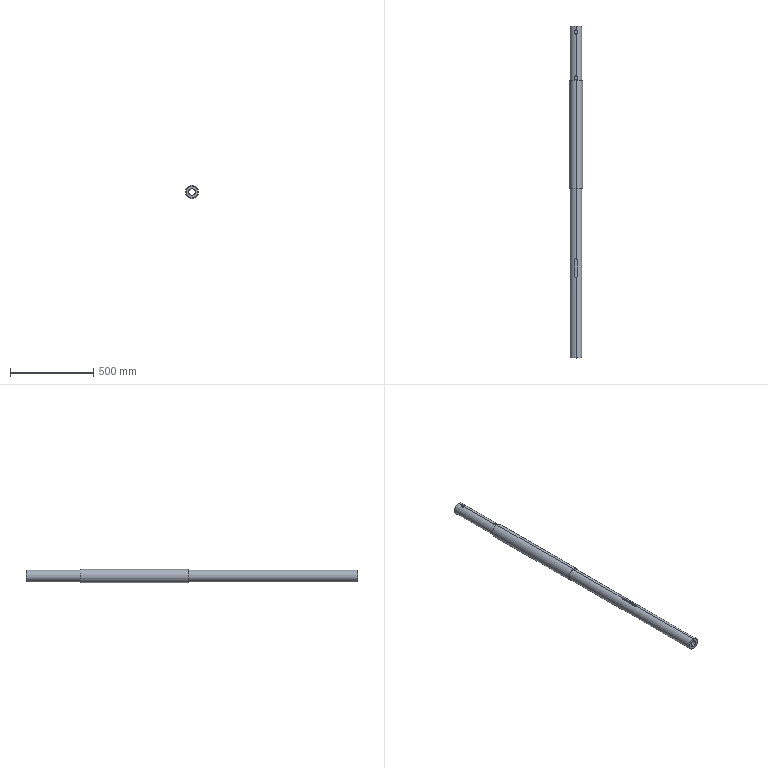Part | SolidWorks | features BaseBody 1 | 1 solid | 31 faces | box 80 x 1994 x 80 mm | volume 5902452 mm3 | cylinder 14 | plane 13 | cone 4 | commonest cylinder face diameters 14 x6 70 x4 40 x2 80 x2
STEP:
#1=CARTESIAN_POINT('',(0.,1994.06,-34.188));
#2=VERTEX_POINT('',#1);
#3=CARTESIAN_POINT('',(0.,1994.06,34.188));
#4=VERTEX_POINT('',#3);
#5=CARTESIAN_POINT('',(0.,1994.06,0.));
#6=DIRECTION('',(0.,-1.,0.));
#7=DIRECTION('',(0.,0.,-1.));
#8=AXIS2_PLACEMENT_3D('',#5,#6,#7);
#9=CIRCLE('',#8,34.188);
#10=EDGE_CURVE('',#2,#4,#9,.T.);
#11=ORIENTED_EDGE('',*,*,#10,.T.);
#12=CARTESIAN_POINT('',(0.,1993.248,35.));
#13=VERTEX_POINT('',#12);
#14=CARTESIAN_POINT('',(0.,1994.06,34.188));
#15=DIRECTION('',(0.,-0.7071,0.7071));
#16=VECTOR('',#15,1000.);
#17=LINE('',#14,#16);
#18=EDGE_CURVE('',#4,#13,#17,.T.);
#19=ORIENTED_EDGE('',*,*,#18,.T.);
#20=CARTESIAN_POINT('',(0.,1993.248,-35.));
#21=VERTEX_POINT('',#20);
#22=CARTESIAN_POINT('',(0.,1993.248,0.));
#23=DIRECTION('',(0.,-1.,0.));
#24=DIRECTION('',(0.,0.,-1.));
#25=AXIS2_PLACEMENT_3D('',#22,#23,#24);
#26=CIRCLE('',#25,35.);
#27=EDGE_CURVE('',#21,#13,#26,.T.);
#28=ORIENTED_EDGE('',*,*,#27,.F.);
#29=CARTESIAN_POINT('',(0.,1994.06,-34.188));
#30=DIRECTION('',(0.,-0.7071,-0.7071));
#31=VECTOR('',#30,1000.);
#32=LINE('',#29,#31);
#33=EDGE_CURVE('',#2,#21,#32,.T.);
#34=ORIENTED_EDGE('',*,*,#33,.F.);
#35=EDGE_LOOP('',(#11,#19,#28,#34));
#36=FACE_OUTER_BOUND('',#35,.T.);
#37=CARTESIAN_POINT('',(0.,1994.06,0.));
#38=DIRECTION('',(0.,-1.,0.));
#39=DIRECTION('',(0.,0.,-1.));
#40=AXIS2_PLACEMENT_3D('',#37,#38,#39);
#41=CONICAL_SURFACE('',#40,34.188,0.7854);
#42=ADVANCED_FACE('',(#36),#41,.T.);
#43=CARTESIAN_POINT('',(0.,0.,34.188));
#44=VERTEX_POINT('',#43);
#45=CARTESIAN_POINT('',(0.,0.,-34.188));
#46=VERTEX_POINT('',#45);
#47=CARTESIAN_POINT('',(0.,0.,0.));
#48=DIRECTION('',(0.,1.,0.));
#49=DIRECTION('',(0.,0.,1.));
#50=AXIS2_PLACEMENT_3D('',#47,#48,#49);
#51=CIRCLE('',#50,34.188);
#52=EDGE_CURVE('',#44,#46,#51,.T.);
#53=ORIENTED_EDGE('',*,*,#52,.T.);
#54=CARTESIAN_POINT('',(0.,0.812,-35.));
#55=VERTEX_POINT('',#54);
#56=CARTESIAN_POINT('',(0.,0.,-34.188));
#57=DIRECTION('',(0.,0.7071,-0.7071));
#58=VECTOR('',#57,1000.);
#59=LINE('',#56,#58);
#60=EDGE_CURVE('',#46,#55,#59,.T.);
#61=ORIENTED_EDGE('',*,*,#60,.T.);
#62=CARTESIAN_POINT('',(0.,0.812,35.));
#63=VERTEX_POINT('',#62);
#64=CARTESIAN_POINT('',(0.,0.812,0.));
#65=DIRECTION('',(0.,1.,0.));
#66=DIRECTION('',(0.,0.,1.));
#67=AXIS2_PLACEMENT_3D('',#64,#65,#66);
#68=CIRCLE('',#67,35.);
#69=EDGE_CURVE('',#63,#55,#68,.T.);
#70=ORIENTED_EDGE('',*,*,#69,.F.);
#71=CARTESIAN_POINT('',(0.,0.,34.188));
#72=DIRECTION('',(0.,0.7071,0.7071));
#73=VECTOR('',#72,1000.);
#74=LINE('',#71,#73);
#75=EDGE_CURVE('',#44,#63,#74,.T.);
#76=ORIENTED_EDGE('',*,*,#75,.F.);
#77=EDGE_LOOP('',(#53,#61,#70,#76));
#78=FACE_OUTER_BOUND('',#77,.T.);
#79=CARTESIAN_POINT('',(0.,0.,0.));
#80=DIRECTION('',(0.,1.,0.));
#81=DIRECTION('',(0.,0.,1.));
#82=AXIS2_PLACEMENT_3D('',#79,#80,#81);
#83=CONICAL_SURFACE('',#82,34.188,0.7854);
#84=ADVANCED_FACE('',(#78),#83,.T.);
#85=CARTESIAN_POINT('',(0.,1994.06,20.));
#86=VERTEX_POINT('',#85);
#87=CARTESIAN_POINT('',(0.,1994.06,-20.));
#88=VERTEX_POINT('',#87);
#89=CARTESIAN_POINT('',(0.,1994.06,0.));
#90=DIRECTION('',(0.,-1.,0.));
#91=DIRECTION('',(0.,0.,-1.));
#92=AXIS2_PLACEMENT_3D('',#89,#90,#91);
#93=CIRCLE('',#92,20.);
#94=EDGE_CURVE('',#86,#88,#93,.T.);
#95=ORIENTED_EDGE('',*,*,#94,.F.);
#96=CARTESIAN_POINT('',(0.,0.,20.));
#97=VERTEX_POINT('',#96);
#98=CARTESIAN_POINT('',(0.,1994.06,20.));
#99=DIRECTION('',(0.,-1.,0.));
#100=VECTOR('',#99,1000.);
#101=LINE('',#98,#100);
#102=EDGE_CURVE('',#86,#97,#101,.T.);
#103=ORIENTED_EDGE('',*,*,#102,.T.);
#104=CARTESIAN_POINT('',(0.,0.,-20.));
#105=VERTEX_POINT('',#104);
#106=CARTESIAN_POINT('',(0.,0.,0.));
#107=DIRECTION('',(0.,-1.,0.));
#108=DIRECTION('',(0.,0.,-1.));
#109=AXIS2_PLACEMENT_3D('',#106,#107,#108);
#110=CIRCLE('',#109,20.);
#111=EDGE_CURVE('',#97,#105,#110,.T.);
#112=ORIENTED_EDGE('',*,*,#111,.T.);
#113=CARTESIAN_POINT('',(0.,1994.06,-20.));
#114=DIRECTION('',(0.,-1.,0.));
#115=VECTOR('',#114,1000.);
#116=LINE('',#113,#115);
#117=EDGE_CURVE('',#88,#105,#116,.T.);
#118=ORIENTED_EDGE('',*,*,#117,.F.);
#119=EDGE_LOOP('',(#95,#103,#112,#118));
#120=FACE_OUTER_BOUND('',#119,.T.);
#121=CARTESIAN_POINT('',(0.,1994.06,0.));
#122=DIRECTION('',(0.,-1.,0.));
#123=DIRECTION('',(0.,0.,-1.));
#124=AXIS2_PLACEMENT_3D('',#121,#122,#123);
#125=CYLINDRICAL_SURFACE('',#124,20.);
#126=ADVANCED_FACE('',(#120),#125,.F.);
#127=ORIENTED_EDGE('',*,*,#27,.T.);
#128=CARTESIAN_POINT('',(0.,1970.58,35.));
#129=VERTEX_POINT('',#128);
#130=CARTESIAN_POINT('',(0.,1994.06,35.));
#131=DIRECTION('',(0.,-1.,0.));
#132=VECTOR('',#131,1000.);
#133=LINE('',#130,#132);
#134=EDGE_CURVE('',#13,#129,#133,.T.);
#135=ORIENTED_EDGE('',*,*,#134,.T.);
#136=CARTESIAN_POINT('',(7.,1963.58,34.293));
#137=VERTEX_POINT('',#136);
#138=CARTESIAN_POINT('',(0.,1970.58,35.));
#139=CARTESIAN_POINT('',(0.4575,1970.58,35.));
#140=CARTESIAN_POINT('',(0.9224,1970.534,34.991));
#141=CARTESIAN_POINT('',(1.82,1970.355,34.956));
#142=CARTESIAN_POINT('',(2.257,1970.222,34.93));
#143=CARTESIAN_POINT('',(2.893,1969.958,34.881));
#144=CARTESIAN_POINT('',(3.103,1969.859,34.863));
#145=CARTESIAN_POINT('',(3.507,1969.643,34.824));
#146=CARTESIAN_POINT('',(3.702,1969.525,34.804));
#147=CARTESIAN_POINT('',(4.269,1969.146,34.741));
#148=CARTESIAN_POINT('',(4.624,1968.855,34.695));
#149=CARTESIAN_POINT('',(5.274,1968.205,34.602));
#150=CARTESIAN_POINT('',(5.563,1967.853,34.556));
#151=CARTESIAN_POINT('',(5.943,1967.286,34.492));
#152=CARTESIAN_POINT('',(6.061,1967.09,34.471));
#153=CARTESIAN_POINT('',(6.278,1966.685,34.433));
#154=CARTESIAN_POINT('',(6.377,1966.476,34.414));
#155=CARTESIAN_POINT('',(6.64,1965.842,34.365));
#156=CARTESIAN_POINT('',(6.773,1965.406,34.339));
#157=CARTESIAN_POINT('',(6.953,1964.507,34.302));
#158=CARTESIAN_POINT('',(7.,1964.043,34.293));
#159=CARTESIAN_POINT('',(7.,1963.58,34.293));
#160=B_SPLINE_CURVE_WITH_KNOTS('',3,(#138,#139,#140,#141,#142,#143,#144,#145,#146,#147,#148,#149,#150,#151,#152,#153,#154,#155,#156,#157,#158,#159),.UNSPECIFIED.,.F.,.F.,(4,2,2,2,2,2,2,2,2,2,4),(0.01097,0.01234,0.01371,0.0144,0.01508,0.01645,0.01782,0.01851,0.01919,0.02056,0.02193),.UNSPECIFIED.);
#161=EDGE_CURVE('',#129,#137,#160,.T.);
#162=ORIENTED_EDGE('',*,*,#161,.T.);
#163=CARTESIAN_POINT('',(7.,1951.55,34.293));
#164=VERTEX_POINT('',#163);
#165=CARTESIAN_POINT('',(7.,1994.06,34.293));
#166=DIRECTION('',(0.,-1.,0.));
#167=VECTOR('',#166,1000.);
#168=LINE('',#165,#167);
#169=EDGE_CURVE('',#137,#164,#168,.T.);
#170=ORIENTED_EDGE('',*,*,#169,.T.);
#171=CARTESIAN_POINT('',(0.,1944.55,35.));
#172=VERTEX_POINT('',#171);
#173=CARTESIAN_POINT('',(7.,1951.55,34.293));
#174=CARTESIAN_POINT('',(7.,1951.086,34.293));
#175=CARTESIAN_POINT('',(6.954,1950.63,34.302));
#176=CARTESIAN_POINT('',(6.82,1949.958,34.329));
#177=CARTESIAN_POINT('',(6.765,1949.736,34.34));
#178=CARTESIAN_POINT('',(6.631,1949.295,34.366));
#179=CARTESIAN_POINT('',(6.552,1949.077,34.381));
#180=CARTESIAN_POINT('',(6.288,1948.441,34.431));
#181=CARTESIAN_POINT('',(6.073,1948.039,34.47));
#182=CARTESIAN_POINT('',(5.692,1947.469,34.534));
#183=CARTESIAN_POINT('',(5.554,1947.284,34.557));
#184=CARTESIAN_POINT('',(5.262,1946.928,34.602));
#185=CARTESIAN_POINT('',(5.109,1946.759,34.626));
#186=CARTESIAN_POINT('',(4.625,1946.276,34.695));
#187=CARTESIAN_POINT('',(4.274,1945.987,34.74));
#188=CARTESIAN_POINT('',(3.7,1945.603,34.804));
#189=CARTESIAN_POINT('',(3.502,1945.484,34.825));
#190=CARTESIAN_POINT('',(3.098,1945.269,34.863));
#191=CARTESIAN_POINT('',(2.686,1945.074,34.899));
#192=CARTESIAN_POINT('',(2.256,1944.919,34.928));
#193=CARTESIAN_POINT('',(1.817,1944.786,34.954));
#194=CARTESIAN_POINT('',(1.591,1944.729,34.965));
#195=CARTESIAN_POINT('',(0.9131,1944.595,34.991));
#196=CARTESIAN_POINT('',(0.458,1944.55,35.));
#197=CARTESIAN_POINT('',(0.,1944.55,35.));
#198=B_SPLINE_CURVE_WITH_KNOTS('',3,(#173,#174,#175,#176,#177,#178,#179,#180,#181,#182,#183,#184,#185,#186,#187,#188,#189,#190,#191,#192,#193,#194,#195,#196,#197),.UNSPECIFIED.,.F.,.F.,(4,2,2,2,2,2,2,2,2,1,2,2,4),(0.,0.001372,0.002057,0.002743,0.004115,0.004801,0.005486,0.006858,0.007544,0.00823,0.008916,0.009601,0.01097),.UNSPECIFIED.);
#199=EDGE_CURVE('',#164,#172,#198,.T.);
#200=ORIENTED_EDGE('',*,*,#199,.T.);
#201=CARTESIAN_POINT('',(0.,1695.09,35.));
#202=VERTEX_POINT('',#201);
#203=CARTESIAN_POINT('',(0.,1994.06,35.));
#204=DIRECTION('',(0.,-1.,0.));
#205=VECTOR('',#204,1000.);
#206=LINE('',#203,#205);
#207=EDGE_CURVE('',#172,#202,#206,.T.);
#208=ORIENTED_EDGE('',*,*,#207,.T.);
#209=CARTESIAN_POINT('',(7.,1688.09,34.293));
#210=VERTEX_POINT('',#209);
#211=CARTESIAN_POINT('',(0.,1695.09,35.));
#212=CARTESIAN_POINT('',(0.4575,1695.09,35.));
#213=CARTESIAN_POINT('',(0.9224,1695.044,34.991));
#214=CARTESIAN_POINT('',(1.82,1694.865,34.956));
#215=CARTESIAN_POINT('',(2.257,1694.732,34.93));
#216=CARTESIAN_POINT('',(2.893,1694.468,34.881));
#217=CARTESIAN_POINT('',(3.103,1694.369,34.863));
#218=CARTESIAN_POINT('',(3.507,1694.153,34.824));
#219=CARTESIAN_POINT('',(3.702,1694.035,34.804));
#220=CARTESIAN_POINT('',(4.269,1693.656,34.741));
#221=CARTESIAN_POINT('',(4.624,1693.365,34.695));
#222=CARTESIAN_POINT('',(5.274,1692.715,34.602));
#223=CARTESIAN_POINT('',(5.563,1692.363,34.556));
#224=CARTESIAN_POINT('',(5.943,1691.796,34.492));
#225=CARTESIAN_POINT('',(6.061,1691.6,34.471));
#226=CARTESIAN_POINT('',(6.278,1691.195,34.433));
#227=CARTESIAN_POINT('',(6.377,1690.986,34.414));
#228=CARTESIAN_POINT('',(6.64,1690.352,34.365));
#229=CARTESIAN_POINT('',(6.773,1689.916,34.339));
#230=CARTESIAN_POINT('',(6.953,1689.017,34.302));
#231=CARTESIAN_POINT('',(7.,1688.553,34.293));
#232=CARTESIAN_POINT('',(7.,1688.09,34.293));
#233=B_SPLINE_CURVE_WITH_KNOTS('',3,(#211,#212,#213,#214,#215,#216,#217,#218,#219,#220,#221,#222,#223,#224,#225,#226,#227,#228,#229,#230,#231,#232),.UNSPECIFIED.,.F.,.F.,(4,2,2,2,2,2,2,2,2,2,4),(0.01097,0.01234,0.01371,0.0144,0.01508,0.01645,0.01782,0.01851,0.01919,0.02056,0.02193),.UNSPECIFIED.);
#234=EDGE_CURVE('',#202,#210,#233,.T.);
#235=ORIENTED_EDGE('',*,*,#234,.T.);
#236=CARTESIAN_POINT('',(7.,1676.06,34.293));
#237=VERTEX_POINT('',#236);
#238=CARTESIAN_POINT('',(7.,1994.06,34.293));
#239=DIRECTION('',(0.,-1.,0.));
#240=VECTOR('',#239,1000.);
#241=LINE('',#238,#240);
#242=EDGE_CURVE('',#210,#237,#241,.T.);
#243=ORIENTED_EDGE('',*,*,#242,.T.);
#244=CARTESIAN_POINT('',(0.,1669.06,35.));
#245=VERTEX_POINT('',#244);
#246=CARTESIAN_POINT('',(7.,1676.06,34.293));
#247=CARTESIAN_POINT('',(7.,1675.596,34.293));
#248=CARTESIAN_POINT('',(6.954,1675.14,34.302));
#249=CARTESIAN_POINT('',(6.82,1674.468,34.329));
#250=CARTESIAN_POINT('',(6.765,1674.246,34.34));
#251=CARTESIAN_POINT('',(6.631,1673.805,34.366));
#252=CARTESIAN_POINT('',(6.552,1673.587,34.381));
#253=CARTESIAN_POINT('',(6.288,1672.951,34.431));
#254=CARTESIAN_POINT('',(6.073,1672.549,34.47));
#255=CARTESIAN_POINT('',(5.692,1671.979,34.534));
#256=CARTESIAN_POINT('',(5.554,1671.794,34.557));
#257=CARTESIAN_POINT('',(5.262,1671.438,34.602));
#258=CARTESIAN_POINT('',(5.109,1671.269,34.626));
#259=CARTESIAN_POINT('',(4.625,1670.786,34.695));
#260=CARTESIAN_POINT('',(4.274,1670.497,34.74));
#261=CARTESIAN_POINT('',(3.7,1670.113,34.804));
#262=CARTESIAN_POINT('',(3.502,1669.994,34.825));
#263=CARTESIAN_POINT('',(3.098,1669.779,34.863));
#264=CARTESIAN_POINT('',(2.686,1669.584,34.899));
#265=CARTESIAN_POINT('',(2.256,1669.429,34.928));
#266=CARTESIAN_POINT('',(1.817,1669.296,34.954));
#267=CARTESIAN_POINT('',(1.591,1669.239,34.965));
#268=CARTESIAN_POINT('',(0.9131,1669.105,34.991));
#269=CARTESIAN_POINT('',(0.458,1669.06,35.));
#270=CARTESIAN_POINT('',(0.,1669.06,35.));
#271=B_SPLINE_CURVE_WITH_KNOTS('',3,(#246,#247,#248,#249,#250,#251,#252,#253,#254,#255,#256,#257,#258,#259,#260,#261,#262,#263,#264,#265,#266,#267,#268,#269,#270),.UNSPECIFIED.,.F.,.F.,(4,2,2,2,2,2,2,2,2,1,2,2,4),(0.,0.001372,0.002057,0.002743,0.004115,0.004801,0.005486,0.006858,0.007544,0.00823,0.008916,0.009601,0.01097),.UNSPECIFIED.);
#272=EDGE_CURVE('',#237,#245,#271,.T.);
#273=ORIENTED_EDGE('',*,*,#272,.T.);
#274=CARTESIAN_POINT('',(0.,1669.06,-35.));
#275=VERTEX_POINT('',#274);
#276=CARTESIAN_POINT('',(0.,1669.06,0.));
#277=DIRECTION('',(0.,1.,0.));
#278=DIRECTION('',(0.,0.,1.));
#279=AXIS2_PLACEMENT_3D('',#276,#277,#278);
#280=CIRCLE('',#279,35.);
#281=EDGE_CURVE('',#245,#275,#280,.T.);
#282=ORIENTED_EDGE('',*,*,#281,.T.);
#283=CARTESIAN_POINT('',(0.,1994.06,-35.));
#284=DIRECTION('',(0.,-1.,0.));
#285=VECTOR('',#284,1000.);
#286=LINE('',#283,#285);
#287=EDGE_CURVE('',#21,#275,#286,.T.);
#288=ORIENTED_EDGE('',*,*,#287,.F.);
#289=EDGE_LOOP('',(#127,#135,#162,#170,#200,#208,#235,#243,#273,#282,#288));
#290=FACE_OUTER_BOUND('',#289,.T.);
#291=CARTESIAN_POINT('',(0.,1994.06,0.));
#292=DIRECTION('',(0.,-1.,0.));
#293=DIRECTION('',(0.,0.,-1.));
#294=AXIS2_PLACEMENT_3D('',#291,#292,#293);
#295=CYLINDRICAL_SURFACE('',#294,35.);
#296=ADVANCED_FACE('',(#290),#295,.T.);
#297=CARTESIAN_POINT('',(0.,1669.06,40.));
#298=VERTEX_POINT('',#297);
#299=CARTESIAN_POINT('',(0.,1669.06,-40.));
#300=VERTEX_POINT('',#299);
#301=CARTESIAN_POINT('',(0.,1669.06,0.));
#302=DIRECTION('',(0.,1.,0.));
#303=DIRECTION('',(0.,0.,1.));
#304=AXIS2_PLACEMENT_3D('',#301,#302,#303);
#305=CIRCLE('',#304,40.);
#306=EDGE_CURVE('',#298,#300,#305,.T.);
#307=ORIENTED_EDGE('',*,*,#306,.F.);
#308=CARTESIAN_POINT('',(0.,1020.,40.));
#309=VERTEX_POINT('',#308);
#310=CARTESIAN_POINT('',(0.,1669.06,40.));
#311=DIRECTION('',(0.,-1.,0.));
#312=VECTOR('',#311,1000.);
#313=LINE('',#310,#312);
#314=EDGE_CURVE('',#298,#309,#313,.T.);
#315=ORIENTED_EDGE('',*,*,#314,.T.);
#316=CARTESIAN_POINT('',(0.,1020.,-40.));
#317=VERTEX_POINT('',#316);
#318=CARTESIAN_POINT('',(0.,1020.,0.));
#319=DIRECTION('',(0.,1.,0.));
#320=DIRECTION('',(0.,0.,1.));
#321=AXIS2_PLACEMENT_3D('',#318,#319,#320);
#322=CIRCLE('',#321,40.);
#323=EDGE_CURVE('',#309,#317,#322,.T.);
#324=ORIENTED_EDGE('',*,*,#323,.T.);
#325=CARTESIAN_POINT('',(0.,1669.06,-40.));
#326=DIRECTION('',(0.,-1.,0.));
#327=VECTOR('',#326,1000.);
#328=LINE('',#325,#327);
#329=EDGE_CURVE('',#300,#317,#328,.T.);
#330=ORIENTED_EDGE('',*,*,#329,.F.);
#331=EDGE_LOOP('',(#307,#315,#324,#330));
#332=FACE_OUTER_BOUND('',#331,.T.);
#333=CARTESIAN_POINT('',(0.,1669.06,0.));
#334=DIRECTION('',(0.,-1.,0.));
#335=DIRECTION('',(0.,0.,-1.));
#336=AXIS2_PLACEMENT_3D('',#333,#334,#335);
#337=CYLINDRICAL_SURFACE('',#336,40.);
#338=ADVANCED_FACE('',(#332),#337,.T.);
#339=CARTESIAN_POINT('',(0.,1020.,35.));
#340=VERTEX_POINT('',#339);
#341=CARTESIAN_POINT('',(0.,1020.,-35.));
#342=VERTEX_POINT('',#341);
#343=CARTESIAN_POINT('',(0.,1020.,0.));
#344=DIRECTION('',(0.,1.,0.));
#345=DIRECTION('',(0.,0.,1.));
#346=AXIS2_PLACEMENT_3D('',#343,#344,#345);
#347=CIRCLE('',#346,35.);
#348=EDGE_CURVE('',#340,#342,#347,.T.);
#349=ORIENTED_EDGE('',*,*,#348,.F.);
#350=CARTESIAN_POINT('',(0.,597.,35.));
#351=VERTEX_POINT('',#350);
#352=CARTESIAN_POINT('',(0.,1020.,35.));
#353=DIRECTION('',(0.,-1.,0.));
#354=VECTOR('',#353,1000.);
#355=LINE('',#352,#354);
#356=EDGE_CURVE('',#340,#351,#355,.T.);
#357=ORIENTED_EDGE('',*,*,#356,.T.);
#358=CARTESIAN_POINT('',(7.,590.,34.293));
#359=VERTEX_POINT('',#358);
#360=CARTESIAN_POINT('',(0.,597.,35.));
#361=CARTESIAN_POINT('',(0.4575,597.,35.));
#362=CARTESIAN_POINT('',(0.9224,596.954,34.991));
#363=CARTESIAN_POINT('',(1.82,596.775,34.956));
#364=CARTESIAN_POINT('',(2.257,596.642,34.93));
#365=CARTESIAN_POINT('',(2.893,596.378,34.881));
#366=CARTESIAN_POINT('',(3.103,596.279,34.863));
#367=CARTESIAN_POINT('',(3.507,596.063,34.824));
#368=CARTESIAN_POINT('',(3.702,595.945,34.804));
#369=CARTESIAN_POINT('',(4.269,595.566,34.741));
#370=CARTESIAN_POINT('',(4.624,595.275,34.695));
#371=CARTESIAN_POINT('',(5.274,594.625,34.602));
#372=CARTESIAN_POINT('',(5.563,594.273,34.556));
#373=CARTESIAN_POINT('',(5.943,593.706,34.492));
#374=CARTESIAN_POINT('',(6.061,593.51,34.471));
#375=CARTESIAN_POINT('',(6.278,593.105,34.433));
#376=CARTESIAN_POINT('',(6.377,592.896,34.414));
#377=CARTESIAN_POINT('',(6.64,592.262,34.365));
#378=CARTESIAN_POINT('',(6.773,591.826,34.339));
#379=CARTESIAN_POINT('',(6.953,590.927,34.302));
#380=CARTESIAN_POINT('',(7.,590.463,34.293));
#381=CARTESIAN_POINT('',(7.,590.,34.293));
#382=B_SPLINE_CURVE_WITH_KNOTS('',3,(#360,#361,#362,#363,#364,#365,#366,#367,#368,#369,#370,#371,#372,#373,#374,#375,#376,#377,#378,#379,#380,#381),.UNSPECIFIED.,.F.,.F.,(4,2,2,2,2,2,2,2,2,2,4),(0.01097,0.01234,0.01371,0.0144,0.01508,0.01645,0.01782,0.01851,0.01919,0.02056,0.02193),.UNSPECIFIED.);
#383=EDGE_CURVE('',#351,#359,#382,.T.);
#384=ORIENTED_EDGE('',*,*,#383,.T.);
#385=CARTESIAN_POINT('',(7.,490.,34.293));
#386=VERTEX_POINT('',#385);
#387=CARTESIAN_POINT('',(7.,1020.,34.293));
#388=DIRECTION('',(0.,-1.,0.));
#389=VECTOR('',#388,1000.);
#390=LINE('',#387,#389);
#391=EDGE_CURVE('',#359,#386,#390,.T.);
#392=ORIENTED_EDGE('',*,*,#391,.T.);
#393=CARTESIAN_POINT('',(0.,483.,35.));
#394=VERTEX_POINT('',#393);
#395=CARTESIAN_POINT('',(7.,490.,34.293));
#396=CARTESIAN_POINT('',(7.,489.536,34.293));
#397=CARTESIAN_POINT('',(6.954,489.08,34.302));
#398=CARTESIAN_POINT('',(6.82,488.408,34.329));
#399=CARTESIAN_POINT('',(6.765,488.186,34.34));
#400=CARTESIAN_POINT('',(6.631,487.745,34.366));
#401=CARTESIAN_POINT('',(6.552,487.527,34.381));
#402=CARTESIAN_POINT('',(6.288,486.891,34.431));
#403=CARTESIAN_POINT('',(6.073,486.489,34.47));
#404=CARTESIAN_POINT('',(5.692,485.919,34.534));
#405=CARTESIAN_POINT('',(5.554,485.734,34.557));
#406=CARTESIAN_POINT('',(5.262,485.378,34.602));
#407=CARTESIAN_POINT('',(5.109,485.209,34.626));
#408=CARTESIAN_POINT('',(4.625,484.726,34.695));
#409=CARTESIAN_POINT('',(4.274,484.437,34.74));
#410=CARTESIAN_POINT('',(3.7,484.053,34.804));
#411=CARTESIAN_POINT('',(3.502,483.934,34.825));
#412=CARTESIAN_POINT('',(3.098,483.719,34.863));
#413=CARTESIAN_POINT('',(2.686,483.524,34.899));
#414=CARTESIAN_POINT('',(2.256,483.369,34.928));
#415=CARTESIAN_POINT('',(1.817,483.236,34.954));
#416=CARTESIAN_POINT('',(1.591,483.179,34.965));
#417=CARTESIAN_POINT('',(0.9131,483.045,34.991));
#418=CARTESIAN_POINT('',(0.458,483.,35.));
#419=CARTESIAN_POINT('',(0.,483.,35.));
#420=B_SPLINE_CURVE_WITH_KNOTS('',3,(#395,#396,#397,#398,#399,#400,#401,#402,#403,#404,#405,#406,#407,#408,#409,#410,#411,#412,#413,#414,#415,#416,#417,#418,#419),.UNSPECIFIED.,.F.,.F.,(4,2,2,2,2,2,2,2,2,1,2,2,4),(0.,0.001372,0.002057,0.002743,0.004115,0.004801,0.005486,0.006858,0.007544,0.00823,0.008916,0.009601,0.01097),.UNSPECIFIED.);
#421=EDGE_CURVE('',#386,#394,#420,.T.);
#422=ORIENTED_EDGE('',*,*,#421,.T.);
#423=CARTESIAN_POINT('',(0.,1020.,35.));
#424=DIRECTION('',(0.,-1.,0.));
#425=VECTOR('',#424,1000.);
#426=LINE('',#423,#425);
#427=EDGE_CURVE('',#394,#63,#426,.T.);
#428=ORIENTED_EDGE('',*,*,#427,.T.);
#429=ORIENTED_EDGE('',*,*,#69,.T.);
#430=CARTESIAN_POINT('',(0.,1020.,-35.));
#431=DIRECTION('',(0.,-1.,0.));
#432=VECTOR('',#431,1000.);
#433=LINE('',#430,#432);
#434=EDGE_CURVE('',#342,#55,#433,.T.);
#435=ORIENTED_EDGE('',*,*,#434,.F.);
#436=EDGE_LOOP('',(#349,#357,#384,#392,#422,#428,#429,#435));
#437=FACE_OUTER_BOUND('',#436,.T.);
#438=CARTESIAN_POINT('',(0.,1020.,0.));
#439=DIRECTION('',(0.,-1.,0.));
#440=DIRECTION('',(0.,0.,-1.));
#441=AXIS2_PLACEMENT_3D('',#438,#439,#440);
#442=CYLINDRICAL_SURFACE('',#441,35.);
#443=ADVANCED_FACE('',(#437),#442,.T.);
#444=CARTESIAN_POINT('',(0.,1994.06,0.));
#445=DIRECTION('',(0.,-1.,0.));
#446=DIRECTION('',(0.,0.,-1.));
#447=AXIS2_PLACEMENT_3D('',#444,#445,#446);
#448=CIRCLE('',#447,20.);
#449=EDGE_CURVE('',#88,#86,#448,.T.);
#450=ORIENTED_EDGE('',*,*,#449,.T.);
#451=ORIENTED_EDGE('',*,*,#94,.T.);
#452=EDGE_LOOP('',(#450,#451));
#453=FACE_BOUND('',#452,.T.);
#454=ORIENTED_EDGE('',*,*,#10,.F.);
#455=CARTESIAN_POINT('',(0.,1994.06,0.));
#456=DIRECTION('',(0.,-1.,0.));
#457=DIRECTION('',(0.,0.,-1.));
#458=AXIS2_PLACEMENT_3D('',#455,#456,#457);
#459=CIRCLE('',#458,34.188);
#460=EDGE_CURVE('',#4,#2,#459,.T.);
#461=ORIENTED_EDGE('',*,*,#460,.F.);
#462=EDGE_LOOP('',(#454,#461));
#463=FACE_OUTER_BOUND('',#462,.T.);
#464=CARTESIAN_POINT('',(0.,1994.06,0.));
#465=DIRECTION('',(0.,1.,0.));
#466=DIRECTION('',(0.,0.,1.));
#467=AXIS2_PLACEMENT_3D('',#464,#465,#466);
#468=PLANE('',#467);
#469=ADVANCED_FACE('',(#453,#463),#468,.T.);
#470=CARTESIAN_POINT('',(0.,0.,0.));
#471=DIRECTION('',(0.,-1.,0.));
#472=DIRECTION('',(0.,0.,-1.));
#473=AXIS2_PLACEMENT_3D('',#470,#471,#472);
#474=CIRCLE('',#473,20.);
#475=EDGE_CURVE('',#105,#97,#474,.T.);
#476=ORIENTED_EDGE('',*,*,#475,.F.);
#477=ORIENTED_EDGE('',*,*,#111,.F.);
#478=EDGE_LOOP('',(#476,#477));
#479=FACE_BOUND('',#478,.T.);
#480=ORIENTED_EDGE('',*,*,#52,.F.);
#481=CARTESIAN_POINT('',(0.,0.,0.));
#482=DIRECTION('',(0.,1.,0.));
#483=DIRECTION('',(0.,0.,1.));
#484=AXIS2_PLACEMENT_3D('',#481,#482,#483);
#485=CIRCLE('',#484,34.188);
#486=EDGE_CURVE('',#46,#44,#485,.T.);
#487=ORIENTED_EDGE('',*,*,#486,.F.);
#488=EDGE_LOOP('',(#480,#487));
#489=FACE_OUTER_BOUND('',#488,.T.);
#490=CARTESIAN_POINT('',(0.,0.,0.));
#491=DIRECTION('',(0.,1.,0.));
#492=DIRECTION('',(0.,0.,1.));
#493=AXIS2_PLACEMENT_3D('',#490,#491,#492);
#494=PLANE('',#493);
#495=ADVANCED_FACE('',(#479,#489),#494,.F.);
#496=ORIENTED_EDGE('',*,*,#356,.F.);
#497=CARTESIAN_POINT('',(0.,1020.,0.));
#498=DIRECTION('',(0.,1.,0.));
#499=DIRECTION('',(0.,0.,1.));
#500=AXIS2_PLACEMENT_3D('',#497,#498,#499);
#501=CIRCLE('',#500,35.);
#502=EDGE_CURVE('',#342,#340,#501,.T.);
#503=ORIENTED_EDGE('',*,*,#502,.F.);
#504=ORIENTED_EDGE('',*,*,#434,.T.);
#505=CARTESIAN_POINT('',(0.,0.812,0.));
#506=DIRECTION('',(0.,1.,0.));
#507=DIRECTION('',(0.,0.,1.));
#508=AXIS2_PLACEMENT_3D('',#505,#506,#507);
#509=CIRCLE('',#508,35.);
#510=EDGE_CURVE('',#55,#63,#509,.T.);
#511=ORIENTED_EDGE('',*,*,#510,.T.);
#512=ORIENTED_EDGE('',*,*,#427,.F.);
#513=CARTESIAN_POINT('',(-7.,490.,34.293));
#514=VERTEX_POINT('',#513);
#515=CARTESIAN_POINT('',(0.,483.,35.));
#516=CARTESIAN_POINT('',(-0.4575,483.,35.));
#517=CARTESIAN_POINT('',(-0.9224,483.046,34.991));
#518=CARTESIAN_POINT('',(-1.82,483.225,34.956));
#519=CARTESIAN_POINT('',(-2.257,483.358,34.93));
#520=CARTESIAN_POINT('',(-2.893,483.622,34.881));
#521=CARTESIAN_POINT('',(-3.103,483.721,34.863));
#522=CARTESIAN_POINT('',(-3.507,483.937,34.824));
#523=CARTESIAN_POINT('',(-3.702,484.055,34.804));
#524=CARTESIAN_POINT('',(-4.269,484.434,34.741));
#525=CARTESIAN_POINT('',(-4.624,484.725,34.695));
#526=CARTESIAN_POINT('',(-5.274,485.375,34.602));
#527=CARTESIAN_POINT('',(-5.563,485.727,34.556));
#528=CARTESIAN_POINT('',(-5.943,486.294,34.492));
#529=CARTESIAN_POINT('',(-6.061,486.49,34.471));
#530=CARTESIAN_POINT('',(-6.278,486.895,34.433));
#531=CARTESIAN_POINT('',(-6.377,487.104,34.414));
#532=CARTESIAN_POINT('',(-6.64,487.738,34.365));
#533=CARTESIAN_POINT('',(-6.773,488.174,34.339));
#534=CARTESIAN_POINT('',(-6.953,489.073,34.302));
#535=CARTESIAN_POINT('',(-7.,489.537,34.293));
#536=CARTESIAN_POINT('',(-7.,490.,34.293));
#537=B_SPLINE_CURVE_WITH_KNOTS('',3,(#515,#516,#517,#518,#519,#520,#521,#522,#523,#524,#525,#526,#527,#528,#529,#530,#531,#532,#533,#534,#535,#536),.UNSPECIFIED.,.F.,.F.,(4,2,2,2,2,2,2,2,2,2,4),(0.01097,0.01234,0.01371,0.0144,0.01508,0.01645,0.01782,0.01851,0.01919,0.02056,0.02193),.UNSPECIFIED.);
#538=EDGE_CURVE('',#394,#514,#537,.T.);
#539=ORIENTED_EDGE('',*,*,#538,.T.);
#540=CARTESIAN_POINT('',(-7.,590.,34.293));
#541=VERTEX_POINT('',#540);
#542=CARTESIAN_POINT('',(-7.,1020.,34.293));
#543=DIRECTION('',(0.,1.,0.));
#544=VECTOR('',#543,1000.);
#545=LINE('',#542,#544);
#546=EDGE_CURVE('',#514,#541,#545,.T.);
#547=ORIENTED_EDGE('',*,*,#546,.T.);
#548=CARTESIAN_POINT('',(-7.,590.,34.293));
#549=CARTESIAN_POINT('',(-7.,590.464,34.293));
#550=CARTESIAN_POINT('',(-6.954,590.92,34.302));
#551=CARTESIAN_POINT('',(-6.82,591.592,34.329));
#552=CARTESIAN_POINT('',(-6.765,591.814,34.34));
#553=CARTESIAN_POINT('',(-6.631,592.255,34.366));
#554=CARTESIAN_POINT('',(-6.552,592.473,34.381));
#555=CARTESIAN_POINT('',(-6.288,593.109,34.431));
#556=CARTESIAN_POINT('',(-6.073,593.511,34.47));
#557=CARTESIAN_POINT('',(-5.692,594.081,34.534));
#558=CARTESIAN_POINT('',(-5.554,594.266,34.557));
#559=CARTESIAN_POINT('',(-5.262,594.622,34.602));
#560=CARTESIAN_POINT('',(-5.109,594.791,34.626));
#561=CARTESIAN_POINT('',(-4.625,595.274,34.695));
#562=CARTESIAN_POINT('',(-4.274,595.563,34.74));
#563=CARTESIAN_POINT('',(-3.7,595.947,34.804));
#564=CARTESIAN_POINT('',(-3.502,596.066,34.825));
#565=CARTESIAN_POINT('',(-3.098,596.281,34.863));
#566=CARTESIAN_POINT('',(-2.686,596.476,34.899));
#567=CARTESIAN_POINT('',(-2.256,596.631,34.928));
#568=CARTESIAN_POINT('',(-1.817,596.764,34.954));
#569=CARTESIAN_POINT('',(-1.591,596.821,34.965));
#570=CARTESIAN_POINT('',(-0.9131,596.955,34.991));
#571=CARTESIAN_POINT('',(-0.458,597.,35.));
#572=CARTESIAN_POINT('',(0.,597.,35.));
#573=B_SPLINE_CURVE_WITH_KNOTS('',3,(#548,#549,#550,#551,#552,#553,#554,#555,#556,#557,#558,#559,#560,#561,#562,#563,#564,#565,#566,#567,#568,#569,#570,#571,#572),.UNSPECIFIED.,.F.,.F.,(4,2,2,2,2,2,2,2,2,1,2,2,4),(0.,0.001372,0.002057,0.002743,0.004115,0.004801,0.005486,0.006858,0.007544,0.00823,0.008916,0.009601,0.01097),.UNSPECIFIED.);
#574=EDGE_CURVE('',#541,#351,#573,.T.);
#575=ORIENTED_EDGE('',*,*,#574,.T.);
#576=EDGE_LOOP('',(#496,#503,#504,#511,#512,#539,#547,#575));
#577=FACE_OUTER_BOUND('',#576,.T.);
#578=CARTESIAN_POINT('',(0.,1020.,0.));
#579=DIRECTION('',(0.,-1.,0.));
#580=DIRECTION('',(0.,0.,-1.));
#581=AXIS2_PLACEMENT_3D('',#578,#579,#580);
#582=CYLINDRICAL_SURFACE('',#581,35.);
#583=ADVANCED_FACE('',(#577),#582,.T.);
#584=ORIENTED_EDGE('',*,*,#314,.F.);
#585=CARTESIAN_POINT('',(0.,1669.06,0.));
#586=DIRECTION('',(0.,1.,0.));
#587=DIRECTION('',(0.,0.,1.));
#588=AXIS2_PLACEMENT_3D('',#585,#586,#587);
#589=CIRCLE('',#588,40.);
#590=EDGE_CURVE('',#300,#298,#589,.T.);
#591=ORIENTED_EDGE('',*,*,#590,.F.);
#592=ORIENTED_EDGE('',*,*,#329,.T.);
#593=CARTESIAN_POINT('',(0.,1020.,0.));
#594=DIRECTION('',(0.,1.,0.));
#595=DIRECTION('',(0.,0.,1.));
#596=AXIS2_PLACEMENT_3D('',#593,#594,#595);
#597=CIRCLE('',#596,40.);
#598=EDGE_CURVE('',#317,#309,#597,.T.);
#599=ORIENTED_EDGE('',*,*,#598,.T.);
#600=EDGE_LOOP('',(#584,#591,#592,#599));
#601=FACE_OUTER_BOUND('',#600,.T.);
#602=CARTESIAN_POINT('',(0.,1669.06,0.));
#603=DIRECTION('',(0.,-1.,0.));
#604=DIRECTION('',(0.,0.,-1.));
#605=AXIS2_PLACEMENT_3D('',#602,#603,#604);
#606=CYLINDRICAL_SURFACE('',#605,40.);
#607=ADVANCED_FACE('',(#601),#606,.T.);
#608=ORIENTED_EDGE('',*,*,#281,.F.);
#609=CARTESIAN_POINT('',(0.,1669.06,0.));
#610=DIRECTION('',(0.,1.,0.));
#611=DIRECTION('',(0.,0.,1.));
#612=AXIS2_PLACEMENT_3D('',#609,#610,#611);
#613=CIRCLE('',#612,35.);
#614=EDGE_CURVE('',#275,#245,#613,.T.);
#615=ORIENTED_EDGE('',*,*,#614,.F.);
#616=EDGE_LOOP('',(#608,#615));
#617=FACE_BOUND('',#616,.T.);
#618=ORIENTED_EDGE('',*,*,#590,.T.);
#619=ORIENTED_EDGE('',*,*,#306,.T.);
#620=EDGE_LOOP('',(#618,#619));
#621=FACE_OUTER_BOUND('',#620,.T.);
#622=CARTESIAN_POINT('',(0.,1669.06,0.));
#623=DIRECTION('',(0.,1.,0.));
#624=DIRECTION('',(0.,0.,1.));
#625=AXIS2_PLACEMENT_3D('',#622,#623,#624);
#626=PLANE('',#625);
#627=ADVANCED_FACE('',(#617,#621),#626,.T.);
#628=ORIENTED_EDGE('',*,*,#502,.T.);
#629=ORIENTED_EDGE('',*,*,#348,.T.);
#630=EDGE_LOOP('',(#628,#629));
#631=FACE_BOUND('',#630,.T.);
#632=ORIENTED_EDGE('',*,*,#598,.F.);
#633=ORIENTED_EDGE('',*,*,#323,.F.);
#634=EDGE_LOOP('',(#632,#633));
#635=FACE_OUTER_BOUND('',#634,.T.);
#636=CARTESIAN_POINT('',(0.,1020.,0.));
#637=DIRECTION('',(0.,1.,0.));
#638=DIRECTION('',(0.,0.,1.));
#639=AXIS2_PLACEMENT_3D('',#636,#637,#638);
#640=PLANE('',#639);
#641=ADVANCED_FACE('',(#631,#635),#640,.F.);
#642=ORIENTED_EDGE('',*,*,#134,.F.);
#643=CARTESIAN_POINT('',(0.,1993.248,0.));
#644=DIRECTION('',(0.,-1.,0.));
#645=DIRECTION('',(0.,0.,-1.));
#646=AXIS2_PLACEMENT_3D('',#643,#644,#645);
#647=CIRCLE('',#646,35.);
#648=EDGE_CURVE('',#13,#21,#647,.T.);
#649=ORIENTED_EDGE('',*,*,#648,.T.);
#650=ORIENTED_EDGE('',*,*,#287,.T.);
#651=ORIENTED_EDGE('',*,*,#614,.T.);
#652=CARTESIAN_POINT('',(-7.,1676.06,34.293));
#653=VERTEX_POINT('',#652);
#654=CARTESIAN_POINT('',(0.,1669.06,35.));
#655=CARTESIAN_POINT('',(-0.4575,1669.06,35.));
#656=CARTESIAN_POINT('',(-0.9224,1669.106,34.991));
#657=CARTESIAN_POINT('',(-1.82,1669.285,34.956));
#658=CARTESIAN_POINT('',(-2.257,1669.418,34.93));
#659=CARTESIAN_POINT('',(-2.893,1669.682,34.881));
#660=CARTESIAN_POINT('',(-3.103,1669.781,34.863));
#661=CARTESIAN_POINT('',(-3.507,1669.997,34.824));
#662=CARTESIAN_POINT('',(-3.702,1670.115,34.804));
#663=CARTESIAN_POINT('',(-4.269,1670.494,34.741));
#664=CARTESIAN_POINT('',(-4.624,1670.785,34.695));
#665=CARTESIAN_POINT('',(-5.274,1671.435,34.602));
#666=CARTESIAN_POINT('',(-5.563,1671.787,34.556));
#667=CARTESIAN_POINT('',(-5.943,1672.354,34.492));
#668=CARTESIAN_POINT('',(-6.061,1672.55,34.471));
#669=CARTESIAN_POINT('',(-6.278,1672.955,34.433));
#670=CARTESIAN_POINT('',(-6.377,1673.164,34.414));
#671=CARTESIAN_POINT('',(-6.64,1673.798,34.365));
#672=CARTESIAN_POINT('',(-6.773,1674.234,34.339));
#673=CARTESIAN_POINT('',(-6.953,1675.133,34.302));
#674=CARTESIAN_POINT('',(-7.,1675.597,34.293));
#675=CARTESIAN_POINT('',(-7.,1676.06,34.293));
#676=B_SPLINE_CURVE_WITH_KNOTS('',3,(#654,#655,#656,#657,#658,#659,#660,#661,#662,#663,#664,#665,#666,#667,#668,#669,#670,#671,#672,#673,#674,#675),.UNSPECIFIED.,.F.,.F.,(4,2,2,2,2,2,2,2,2,2,4),(0.01097,0.01234,0.01371,0.0144,0.01508,0.01645,0.01782,0.01851,0.01919,0.02056,0.02193),.UNSPECIFIED.);
#677=EDGE_CURVE('',#245,#653,#676,.T.);
#678=ORIENTED_EDGE('',*,*,#677,.T.);
#679=CARTESIAN_POINT('',(-7.,1688.09,34.293));
#680=VERTEX_POINT('',#679);
#681=CARTESIAN_POINT('',(-7.,1994.06,34.293));
#682=DIRECTION('',(0.,1.,0.));
#683=VECTOR('',#682,1000.);
#684=LINE('',#681,#683);
#685=EDGE_CURVE('',#653,#680,#684,.T.);
#686=ORIENTED_EDGE('',*,*,#685,.T.);
#687=CARTESIAN_POINT('',(-7.,1688.09,34.293));
#688=CARTESIAN_POINT('',(-7.,1688.554,34.293));
#689=CARTESIAN_POINT('',(-6.954,1689.01,34.302));
#690=CARTESIAN_POINT('',(-6.82,1689.682,34.329));
#691=CARTESIAN_POINT('',(-6.765,1689.904,34.34));
#692=CARTESIAN_POINT('',(-6.631,1690.345,34.366));
#693=CARTESIAN_POINT('',(-6.552,1690.563,34.381));
#694=CARTESIAN_POINT('',(-6.288,1691.199,34.431));
#695=CARTESIAN_POINT('',(-6.073,1691.601,34.47));
#696=CARTESIAN_POINT('',(-5.692,1692.171,34.534));
#697=CARTESIAN_POINT('',(-5.554,1692.356,34.557));
#698=CARTESIAN_POINT('',(-5.262,1692.712,34.602));
#699=CARTESIAN_POINT('',(-5.109,1692.881,34.626));
#700=CARTESIAN_POINT('',(-4.625,1693.364,34.695));
#701=CARTESIAN_POINT('',(-4.274,1693.653,34.74));
#702=CARTESIAN_POINT('',(-3.7,1694.037,34.804));
#703=CARTESIAN_POINT('',(-3.502,1694.156,34.825));
#704=CARTESIAN_POINT('',(-3.098,1694.371,34.863));
#705=CARTESIAN_POINT('',(-2.686,1694.566,34.899));
#706=CARTESIAN_POINT('',(-2.256,1694.721,34.928));
#707=CARTESIAN_POINT('',(-1.817,1694.854,34.954));
#708=CARTESIAN_POINT('',(-1.591,1694.911,34.965));
#709=CARTESIAN_POINT('',(-0.9131,1695.045,34.991));
#710=CARTESIAN_POINT('',(-0.458,1695.09,35.));
#711=CARTESIAN_POINT('',(0.,1695.09,35.));
#712=B_SPLINE_CURVE_WITH_KNOTS('',3,(#687,#688,#689,#690,#691,#692,#693,#694,#695,#696,#697,#698,#699,#700,#701,#702,#703,#704,#705,#706,#707,#708,#709,#710,#711),.UNSPECIFIED.,.F.,.F.,(4,2,2,2,2,2,2,2,2,1,2,2,4),(0.,0.001372,0.002057,0.002743,0.004115,0.004801,0.005486,0.006858,0.007544,0.00823,0.008916,0.009601,0.01097),.UNSPECIFIED.);
#713=EDGE_CURVE('',#680,#202,#712,.T.);
#714=ORIENTED_EDGE('',*,*,#713,.T.);
#715=ORIENTED_EDGE('',*,*,#207,.F.);
#716=CARTESIAN_POINT('',(-7.,1951.55,34.293));
#717=VERTEX_POINT('',#716);
#718=CARTESIAN_POINT('',(0.,1944.55,35.));
#719=CARTESIAN_POINT('',(-0.4575,1944.55,35.));
#720=CARTESIAN_POINT('',(-0.9224,1944.596,34.991));
#721=CARTESIAN_POINT('',(-1.82,1944.775,34.956));
#722=CARTESIAN_POINT('',(-2.257,1944.908,34.93));
#723=CARTESIAN_POINT('',(-2.893,1945.172,34.881));
#724=CARTESIAN_POINT('',(-3.103,1945.271,34.863));
#725=CARTESIAN_POINT('',(-3.507,1945.487,34.824));
#726=CARTESIAN_POINT('',(-3.702,1945.605,34.804));
#727=CARTESIAN_POINT('',(-4.269,1945.984,34.741));
#728=CARTESIAN_POINT('',(-4.624,1946.275,34.695));
#729=CARTESIAN_POINT('',(-5.274,1946.925,34.602));
#730=CARTESIAN_POINT('',(-5.563,1947.277,34.556));
#731=CARTESIAN_POINT('',(-5.943,1947.844,34.492));
#732=CARTESIAN_POINT('',(-6.061,1948.04,34.471));
#733=CARTESIAN_POINT('',(-6.278,1948.445,34.433));
#734=CARTESIAN_POINT('',(-6.377,1948.654,34.414));
#735=CARTESIAN_POINT('',(-6.64,1949.288,34.365));
#736=CARTESIAN_POINT('',(-6.773,1949.724,34.339));
#737=CARTESIAN_POINT('',(-6.953,1950.623,34.302));
#738=CARTESIAN_POINT('',(-7.,1951.087,34.293));
#739=CARTESIAN_POINT('',(-7.,1951.55,34.293));
#740=B_SPLINE_CURVE_WITH_KNOTS('',3,(#718,#719,#720,#721,#722,#723,#724,#725,#726,#727,#728,#729,#730,#731,#732,#733,#734,#735,#736,#737,#738,#739),.UNSPECIFIED.,.F.,.F.,(4,2,2,2,2,2,2,2,2,2,4),(0.01097,0.01234,0.01371,0.0144,0.01508,0.01645,0.01782,0.01851,0.01919,0.02056,0.02193),.UNSPECIFIED.);
#741=EDGE_CURVE('',#172,#717,#740,.T.);
#742=ORIENTED_EDGE('',*,*,#741,.T.);
#743=CARTESIAN_POINT('',(-7.,1963.58,34.293));
#744=VERTEX_POINT('',#743);
#745=CARTESIAN_POINT('',(-7.,1994.06,34.293));
#746=DIRECTION('',(0.,1.,0.));
#747=VECTOR('',#746,1000.);
#748=LINE('',#745,#747);
#749=EDGE_CURVE('',#717,#744,#748,.T.);
#750=ORIENTED_EDGE('',*,*,#749,.T.);
#751=CARTESIAN_POINT('',(-7.,1963.58,34.293));
#752=CARTESIAN_POINT('',(-7.,1964.044,34.293));
#753=CARTESIAN_POINT('',(-6.954,1964.5,34.302));
#754=CARTESIAN_POINT('',(-6.82,1965.172,34.329));
#755=CARTESIAN_POINT('',(-6.765,1965.394,34.34));
#756=CARTESIAN_POINT('',(-6.631,1965.835,34.366));
#757=CARTESIAN_POINT('',(-6.552,1966.053,34.381));
#758=CARTESIAN_POINT('',(-6.288,1966.689,34.431));
#759=CARTESIAN_POINT('',(-6.073,1967.091,34.47));
#760=CARTESIAN_POINT('',(-5.692,1967.661,34.534));
#761=CARTESIAN_POINT('',(-5.554,1967.846,34.557));
#762=CARTESIAN_POINT('',(-5.262,1968.202,34.602));
#763=CARTESIAN_POINT('',(-5.109,1968.371,34.626));
#764=CARTESIAN_POINT('',(-4.625,1968.854,34.695));
#765=CARTESIAN_POINT('',(-4.274,1969.143,34.74));
#766=CARTESIAN_POINT('',(-3.7,1969.527,34.804));
#767=CARTESIAN_POINT('',(-3.502,1969.646,34.825));
#768=CARTESIAN_POINT('',(-3.098,1969.861,34.863));
#769=CARTESIAN_POINT('',(-2.686,1970.056,34.899));
#770=CARTESIAN_POINT('',(-2.256,1970.211,34.928));
#771=CARTESIAN_POINT('',(-1.817,1970.344,34.954));
#772=CARTESIAN_POINT('',(-1.591,1970.401,34.965));
#773=CARTESIAN_POINT('',(-0.9131,1970.535,34.991));
#774=CARTESIAN_POINT('',(-0.458,1970.58,35.));
#775=CARTESIAN_POINT('',(0.,1970.58,35.));
#776=B_SPLINE_CURVE_WITH_KNOTS('',3,(#751,#752,#753,#754,#755,#756,#757,#758,#759,#760,#761,#762,#763,#764,#765,#766,#767,#768,#769,#770,#771,#772,#773,#774,#775),.UNSPECIFIED.,.F.,.F.,(4,2,2,2,2,2,2,2,2,1,2,2,4),(0.,0.001372,0.002057,0.002743,0.004115,0.004801,0.005486,0.006858,0.007544,0.00823,0.008916,0.009601,0.01097),.UNSPECIFIED.);
#777=EDGE_CURVE('',#744,#129,#776,.T.);
#778=ORIENTED_EDGE('',*,*,#777,.T.);
#779=EDGE_LOOP('',(#642,#649,#650,#651,#678,#686,#714,#715,#742,#750,#778));
#780=FACE_OUTER_BOUND('',#779,.T.);
#781=CARTESIAN_POINT('',(0.,1994.06,0.));
#782=DIRECTION('',(0.,-1.,0.));
#783=DIRECTION('',(0.,0.,-1.));
#784=AXIS2_PLACEMENT_3D('',#781,#782,#783);
#785=CYLINDRICAL_SURFACE('',#784,35.);
#786=ADVANCED_FACE('',(#780),#785,.T.);
#787=CARTESIAN_POINT('',(7.,1676.06,21.));
#788=VERTEX_POINT('',#787);
#789=CARTESIAN_POINT('',(7.,1676.06,21.));
#790=DIRECTION('',(0.,0.,1.));
#791=VECTOR('',#790,1000.);
#792=LINE('',#789,#791);
#793=EDGE_CURVE('',#788,#237,#792,.T.);
#794=ORIENTED_EDGE('',*,*,#793,.F.);
#795=CARTESIAN_POINT('',(-7.,1676.06,21.));
#796=VERTEX_POINT('',#795);
#797=CARTESIAN_POINT('',(0.,1676.06,21.));
#798=DIRECTION('',(0.,0.,1.));
#799=DIRECTION('',(1.,0.,0.));
#800=AXIS2_PLACEMENT_3D('',#797,#798,#799);
#801=CIRCLE('',#800,7.);
#802=EDGE_CURVE('',#796,#788,#801,.T.);
#803=ORIENTED_EDGE('',*,*,#802,.F.);
#804=CARTESIAN_POINT('',(-7.,1676.06,21.));
#805=DIRECTION('',(0.,0.,1.));
#806=VECTOR('',#805,1000.);
#807=LINE('',#804,#806);
#808=EDGE_CURVE('',#796,#653,#807,.T.);
#809=ORIENTED_EDGE('',*,*,#808,.T.);
#810=ORIENTED_EDGE('',*,*,#677,.F.);
#811=ORIENTED_EDGE('',*,*,#272,.F.);
#812=EDGE_LOOP('',(#794,#803,#809,#810,#811));
#813=FACE_OUTER_BOUND('',#812,.T.);
#814=CARTESIAN_POINT('',(0.,1676.06,21.));
#815=DIRECTION('',(0.,0.,1.));
#816=DIRECTION('',(1.,0.,0.));
#817=AXIS2_PLACEMENT_3D('',#814,#815,#816);
#818=CYLINDRICAL_SURFACE('',#817,7.);
#819=ADVANCED_FACE('',(#813),#818,.F.);
#820=ORIENTED_EDGE('',*,*,#808,.F.);
#821=CARTESIAN_POINT('',(-7.,1688.09,21.));
#822=VERTEX_POINT('',#821);
#823=CARTESIAN_POINT('',(-7.,1676.06,21.));
#824=DIRECTION('',(0.,-1.,0.));
#825=VECTOR('',#824,1000.);
#826=LINE('',#823,#825);
#827=EDGE_CURVE('',#822,#796,#826,.T.);
#828=ORIENTED_EDGE('',*,*,#827,.F.);
#829=CARTESIAN_POINT('',(-7.,1688.09,21.));
#830=DIRECTION('',(0.,0.,1.));
#831=VECTOR('',#830,1000.);
#832=LINE('',#829,#831);
#833=EDGE_CURVE('',#822,#680,#832,.T.);
#834=ORIENTED_EDGE('',*,*,#833,.T.);
#835=ORIENTED_EDGE('',*,*,#685,.F.);
#836=EDGE_LOOP('',(#820,#828,#834,#835));
#837=FACE_OUTER_BOUND('',#836,.T.);
#838=CARTESIAN_POINT('',(-7.,1676.06,21.));
#839=DIRECTION('',(-1.,0.,0.));
#840=DIRECTION('',(0.,-1.,0.));
#841=AXIS2_PLACEMENT_3D('',#838,#839,#840);
#842=PLANE('',#841);
#843=ADVANCED_FACE('',(#837),#842,.F.);
#844=ORIENTED_EDGE('',*,*,#833,.F.);
#845=CARTESIAN_POINT('',(7.,1688.09,21.));
#846=VERTEX_POINT('',#845);
#847=CARTESIAN_POINT('',(0.,1688.09,21.));
#848=DIRECTION('',(0.,0.,1.));
#849=DIRECTION('',(1.,0.,0.));
#850=AXIS2_PLACEMENT_3D('',#847,#848,#849);
#851=CIRCLE('',#850,7.);
#852=EDGE_CURVE('',#846,#822,#851,.T.);
#853=ORIENTED_EDGE('',*,*,#852,.F.);
#854=CARTESIAN_POINT('',(7.,1688.09,21.));
#855=DIRECTION('',(0.,0.,1.));
#856=VECTOR('',#855,1000.);
#857=LINE('',#854,#856);
#858=EDGE_CURVE('',#846,#210,#857,.T.);
#859=ORIENTED_EDGE('',*,*,#858,.T.);
#860=ORIENTED_EDGE('',*,*,#234,.F.);
#861=ORIENTED_EDGE('',*,*,#713,.F.);
#862=EDGE_LOOP('',(#844,#853,#859,#860,#861));
#863=FACE_OUTER_BOUND('',#862,.T.);
#864=CARTESIAN_POINT('',(0.,1688.09,21.));
#865=DIRECTION('',(0.,0.,1.));
#866=DIRECTION('',(1.,0.,0.));
#867=AXIS2_PLACEMENT_3D('',#864,#865,#866);
#868=CYLINDRICAL_SURFACE('',#867,7.);
#869=ADVANCED_FACE('',(#863),#868,.F.);
#870=ORIENTED_EDGE('',*,*,#858,.F.);
#871=CARTESIAN_POINT('',(7.,1676.06,21.));
#872=DIRECTION('',(0.,1.,0.));
#873=VECTOR('',#872,1000.);
#874=LINE('',#871,#873);
#875=EDGE_CURVE('',#788,#846,#874,.T.);
#876=ORIENTED_EDGE('',*,*,#875,.F.);
#877=ORIENTED_EDGE('',*,*,#793,.T.);
#878=ORIENTED_EDGE('',*,*,#242,.F.);
#879=EDGE_LOOP('',(#870,#876,#877,#878));
#880=FACE_OUTER_BOUND('',#879,.T.);
#881=CARTESIAN_POINT('',(7.,1676.06,21.));
#882=DIRECTION('',(1.,0.,0.));
#883=DIRECTION('',(0.,1.,0.));
#884=AXIS2_PLACEMENT_3D('',#881,#882,#883);
#885=PLANE('',#884);
#886=ADVANCED_FACE('',(#880),#885,.F.);
#887=ORIENTED_EDGE('',*,*,#802,.T.);
#888=ORIENTED_EDGE('',*,*,#875,.T.);
#889=ORIENTED_EDGE('',*,*,#852,.T.);
#890=ORIENTED_EDGE('',*,*,#827,.T.);
#891=EDGE_LOOP('',(#887,#888,#889,#890));
#892=FACE_OUTER_BOUND('',#891,.T.);
#893=CARTESIAN_POINT('',(0.,1676.06,21.));
#894=DIRECTION('',(0.,0.,1.));
#895=DIRECTION('',(1.,0.,0.));
#896=AXIS2_PLACEMENT_3D('',#893,#894,#895);
#897=PLANE('',#896);
#898=ADVANCED_FACE('',(#892),#897,.T.);
#899=CARTESIAN_POINT('',(-7.,1963.58,21.));
#900=VERTEX_POINT('',#899);
#901=CARTESIAN_POINT('',(-7.,1963.58,21.));
#902=DIRECTION('',(0.,0.,1.));
#903=VECTOR('',#902,1000.);
#904=LINE('',#901,#903);
#905=EDGE_CURVE('',#900,#744,#904,.T.);
#906=ORIENTED_EDGE('',*,*,#905,.F.);
#907=CARTESIAN_POINT('',(7.,1963.58,21.));
#908=VERTEX_POINT('',#907);
#909=CARTESIAN_POINT('',(0.,1963.58,21.));
#910=DIRECTION('',(0.,0.,1.));
#911=DIRECTION('',(1.,0.,0.));
#912=AXIS2_PLACEMENT_3D('',#909,#910,#911);
#913=CIRCLE('',#912,7.);
#914=EDGE_CURVE('',#908,#900,#913,.T.);
#915=ORIENTED_EDGE('',*,*,#914,.F.);
#916=CARTESIAN_POINT('',(7.,1963.58,21.));
#917=DIRECTION('',(0.,0.,1.));
#918=VECTOR('',#917,1000.);
#919=LINE('',#916,#918);
#920=EDGE_CURVE('',#908,#137,#919,.T.);
#921=ORIENTED_EDGE('',*,*,#920,.T.);
#922=ORIENTED_EDGE('',*,*,#161,.F.);
#923=ORIENTED_EDGE('',*,*,#777,.F.);
#924=EDGE_LOOP('',(#906,#915,#921,#922,#923));
#925=FACE_OUTER_BOUND('',#924,.T.);
#926=CARTESIAN_POINT('',(0.,1963.58,21.));
#927=DIRECTION('',(0.,0.,1.));
#928=DIRECTION('',(1.,0.,0.));
#929=AXIS2_PLACEMENT_3D('',#926,#927,#928);
#930=CYLINDRICAL_SURFACE('',#929,7.);
#931=ADVANCED_FACE('',(#925),#930,.F.);
#932=ORIENTED_EDGE('',*,*,#920,.F.);
#933=CARTESIAN_POINT('',(7.,1951.55,21.));
#934=VERTEX_POINT('',#933);
#935=CARTESIAN_POINT('',(7.,1963.58,21.));
#936=DIRECTION('',(0.,1.,0.));
#937=VECTOR('',#936,1000.);
#938=LINE('',#935,#937);
#939=EDGE_CURVE('',#934,#908,#938,.T.);
#940=ORIENTED_EDGE('',*,*,#939,.F.);
#941=CARTESIAN_POINT('',(7.,1951.55,21.));
#942=DIRECTION('',(0.,0.,1.));
#943=VECTOR('',#942,1000.);
#944=LINE('',#941,#943);
#945=EDGE_CURVE('',#934,#164,#944,.T.);
#946=ORIENTED_EDGE('',*,*,#945,.T.);
#947=ORIENTED_EDGE('',*,*,#169,.F.);
#948=EDGE_LOOP('',(#932,#940,#946,#947));
#949=FACE_OUTER_BOUND('',#948,.T.);
#950=CARTESIAN_POINT('',(7.,1963.58,21.));
#951=DIRECTION('',(1.,0.,0.));
#952=DIRECTION('',(0.,1.,0.));
#953=AXIS2_PLACEMENT_3D('',#950,#951,#952);
#954=PLANE('',#953);
#955=ADVANCED_FACE('',(#949),#954,.F.);
#956=ORIENTED_EDGE('',*,*,#945,.F.);
#957=CARTESIAN_POINT('',(-7.,1951.55,21.));
#958=VERTEX_POINT('',#957);
#959=CARTESIAN_POINT('',(0.,1951.55,21.));
#960=DIRECTION('',(0.,0.,1.));
#961=DIRECTION('',(1.,0.,0.));
#962=AXIS2_PLACEMENT_3D('',#959,#960,#961);
#963=CIRCLE('',#962,7.);
#964=EDGE_CURVE('',#958,#934,#963,.T.);
#965=ORIENTED_EDGE('',*,*,#964,.F.);
#966=CARTESIAN_POINT('',(-7.,1951.55,21.));
#967=DIRECTION('',(0.,0.,1.));
#968=VECTOR('',#967,1000.);
#969=LINE('',#966,#968);
#970=EDGE_CURVE('',#958,#717,#969,.T.);
#971=ORIENTED_EDGE('',*,*,#970,.T.);
#972=ORIENTED_EDGE('',*,*,#741,.F.);
#973=ORIENTED_EDGE('',*,*,#199,.F.);
#974=EDGE_LOOP('',(#956,#965,#971,#972,#973));
#975=FACE_OUTER_BOUND('',#974,.T.);
#976=CARTESIAN_POINT('',(0.,1951.55,21.));
#977=DIRECTION('',(0.,0.,1.));
#978=DIRECTION('',(1.,0.,0.));
#979=AXIS2_PLACEMENT_3D('',#976,#977,#978);
#980=CYLINDRICAL_SURFACE('',#979,7.);
#981=ADVANCED_FACE('',(#975),#980,.F.);
#982=ORIENTED_EDGE('',*,*,#970,.F.);
#983=CARTESIAN_POINT('',(-7.,1963.58,21.));
#984=DIRECTION('',(0.,-1.,0.));
#985=VECTOR('',#984,1000.);
#986=LINE('',#983,#985);
#987=EDGE_CURVE('',#900,#958,#986,.T.);
#988=ORIENTED_EDGE('',*,*,#987,.F.);
#989=ORIENTED_EDGE('',*,*,#905,.T.);
#990=ORIENTED_EDGE('',*,*,#749,.F.);
#991=EDGE_LOOP('',(#982,#988,#989,#990));
#992=FACE_OUTER_BOUND('',#991,.T.);
#993=CARTESIAN_POINT('',(-7.,1963.58,21.));
#994=DIRECTION('',(-1.,0.,0.));
#995=DIRECTION('',(0.,-1.,0.));
#996=AXIS2_PLACEMENT_3D('',#993,#994,#995);
#997=PLANE('',#996);
#998=ADVANCED_FACE('',(#992),#997,.F.);
#999=ORIENTED_EDGE('',*,*,#914,.T.);
#1000=ORIENTED_EDGE('',*,*,#987,.T.);
#1001=ORIENTED_EDGE('',*,*,#964,.T.);
#1002=ORIENTED_EDGE('',*,*,#939,.T.);
#1003=EDGE_LOOP('',(#999,#1000,#1001,#1002));
#1004=FACE_OUTER_BOUND('',#1003,.T.);
#1005=CARTESIAN_POINT('',(0.,1963.58,21.));
#1006=DIRECTION('',(0.,0.,1.));
#1007=DIRECTION('',(1.,0.,0.));
#1008=AXIS2_PLACEMENT_3D('',#1005,#1006,#1007);
#1009=PLANE('',#1008);
#1010=ADVANCED_FACE('',(#1004),#1009,.T.);
#1011=CARTESIAN_POINT('',(7.,490.,21.));
#1012=VERTEX_POINT('',#1011);
#1013=CARTESIAN_POINT('',(7.,490.,21.));
#1014=DIRECTION('',(0.,0.,1.));
#1015=VECTOR('',#1014,1000.);
#1016=LINE('',#1013,#1015);
#1017=EDGE_CURVE('',#1012,#386,#1016,.T.);
#1018=ORIENTED_EDGE('',*,*,#1017,.F.);
#1019=CARTESIAN_POINT('',(-7.,490.,21.));
#1020=VERTEX_POINT('',#1019);
#1021=CARTESIAN_POINT('',(0.,490.,21.));
#1022=DIRECTION('',(0.,0.,1.));
#1023=DIRECTION('',(1.,0.,0.));
#1024=AXIS2_PLACEMENT_3D('',#1021,#1022,#1023);
#1025=CIRCLE('',#1024,7.);
#1026=EDGE_CURVE('',#1020,#1012,#1025,.T.);
#1027=ORIENTED_EDGE('',*,*,#1026,.F.);
#1028=CARTESIAN_POINT('',(-7.,490.,21.));
#1029=DIRECTION('',(0.,0.,1.));
#1030=VECTOR('',#1029,1000.);
#1031=LINE('',#1028,#1030);
#1032=EDGE_CURVE('',#1020,#514,#1031,.T.);
#1033=ORIENTED_EDGE('',*,*,#1032,.T.);
#1034=ORIENTED_EDGE('',*,*,#538,.F.);
#1035=ORIENTED_EDGE('',*,*,#421,.F.);
#1036=EDGE_LOOP('',(#1018,#1027,#1033,#1034,#1035));
#1037=FACE_OUTER_BOUND('',#1036,.T.);
#1038=CARTESIAN_POINT('',(0.,490.,21.));
#1039=DIRECTION('',(0.,0.,1.));
#1040=DIRECTION('',(1.,0.,0.));
#1041=AXIS2_PLACEMENT_3D('',#1038,#1039,#1040);
#1042=CYLINDRICAL_SURFACE('',#1041,7.);
#1043=ADVANCED_FACE('',(#1037),#1042,.F.);
#1044=ORIENTED_EDGE('',*,*,#1032,.F.);
#1045=CARTESIAN_POINT('',(-7.,590.,21.));
#1046=VERTEX_POINT('',#1045);
#1047=CARTESIAN_POINT('',(-7.,490.,21.));
#1048=DIRECTION('',(0.,-1.,0.));
#1049=VECTOR('',#1048,1000.);
#1050=LINE('',#1047,#1049);
#1051=EDGE_CURVE('',#1046,#1020,#1050,.T.);
#1052=ORIENTED_EDGE('',*,*,#1051,.F.);
#1053=CARTESIAN_POINT('',(-7.,590.,21.));
#1054=DIRECTION('',(0.,0.,1.));
#1055=VECTOR('',#1054,1000.);
#1056=LINE('',#1053,#1055);
#1057=EDGE_CURVE('',#1046,#541,#1056,.T.);
#1058=ORIENTED_EDGE('',*,*,#1057,.T.);
#1059=ORIENTED_EDGE('',*,*,#546,.F.);
#1060=EDGE_LOOP('',(#1044,#1052,#1058,#1059));
#1061=FACE_OUTER_BOUND('',#1060,.T.);
#1062=CARTESIAN_POINT('',(-7.,490.,21.));
#1063=DIRECTION('',(-1.,0.,0.));
#1064=DIRECTION('',(0.,-1.,0.));
#1065=AXIS2_PLACEMENT_3D('',#1062,#1063,#1064);
#1066=PLANE('',#1065);
#1067=ADVANCED_FACE('',(#1061),#1066,.F.);
#1068=ORIENTED_EDGE('',*,*,#1057,.F.);
#1069=CARTESIAN_POINT('',(7.,590.,21.));
#1070=VERTEX_POINT('',#1069);
#1071=CARTESIAN_POINT('',(0.,590.,21.));
#1072=DIRECTION('',(0.,0.,1.));
#1073=DIRECTION('',(1.,0.,0.));
#1074=AXIS2_PLACEMENT_3D('',#1071,#1072,#1073);
#1075=CIRCLE('',#1074,7.);
#1076=EDGE_CURVE('',#1070,#1046,#1075,.T.);
#1077=ORIENTED_EDGE('',*,*,#1076,.F.);
#1078=CARTESIAN_POINT('',(7.,590.,21.));
#1079=DIRECTION('',(0.,0.,1.));
#1080=VECTOR('',#1079,1000.);
#1081=LINE('',#1078,#1080);
#1082=EDGE_CURVE('',#1070,#359,#1081,.T.);
#1083=ORIENTED_EDGE('',*,*,#1082,.T.);
#1084=ORIENTED_EDGE('',*,*,#383,.F.);
#1085=ORIENTED_EDGE('',*,*,#574,.F.);
#1086=EDGE_LOOP('',(#1068,#1077,#1083,#1084,#1085));
#1087=FACE_OUTER_BOUND('',#1086,.T.);
#1088=CARTESIAN_POINT('',(0.,590.,21.));
#1089=DIRECTION('',(0.,0.,1.));
#1090=DIRECTION('',(1.,0.,0.));
#1091=AXIS2_PLACEMENT_3D('',#1088,#1089,#1090);
#1092=CYLINDRICAL_SURFACE('',#1091,7.);
#1093=ADVANCED_FACE('',(#1087),#1092,.F.);
#1094=ORIENTED_EDGE('',*,*,#1082,.F.);
#1095=CARTESIAN_POINT('',(7.,490.,21.));
#1096=DIRECTION('',(0.,1.,0.));
#1097=VECTOR('',#1096,1000.);
#1098=LINE('',#1095,#1097);
#1099=EDGE_CURVE('',#1012,#1070,#1098,.T.);
#1100=ORIENTED_EDGE('',*,*,#1099,.F.);
#1101=ORIENTED_EDGE('',*,*,#1017,.T.);
#1102=ORIENTED_EDGE('',*,*,#391,.F.);
#1103=EDGE_LOOP('',(#1094,#1100,#1101,#1102));
#1104=FACE_OUTER_BOUND('',#1103,.T.);
#1105=CARTESIAN_POINT('',(7.,490.,21.));
#1106=DIRECTION('',(1.,0.,0.));
#1107=DIRECTION('',(0.,1.,0.));
#1108=AXIS2_PLACEMENT_3D('',#1105,#1106,#1107);
#1109=PLANE('',#1108);
#1110=ADVANCED_FACE('',(#1104),#1109,.F.);
#1111=ORIENTED_EDGE('',*,*,#1026,.T.);
#1112=ORIENTED_EDGE('',*,*,#1099,.T.);
#1113=ORIENTED_EDGE('',*,*,#1076,.T.);
#1114=ORIENTED_EDGE('',*,*,#1051,.T.);
#1115=EDGE_LOOP('',(#1111,#1112,#1113,#1114));
#1116=FACE_OUTER_BOUND('',#1115,.T.);
#1117=CARTESIAN_POINT('',(0.,490.,21.));
#1118=DIRECTION('',(0.,0.,1.));
#1119=DIRECTION('',(1.,0.,0.));
#1120=AXIS2_PLACEMENT_3D('',#1117,#1118,#1119);
#1121=PLANE('',#1120);
#1122=ADVANCED_FACE('',(#1116),#1121,.T.);
#1123=ORIENTED_EDGE('',*,*,#102,.F.);
#1124=ORIENTED_EDGE('',*,*,#449,.F.);
#1125=ORIENTED_EDGE('',*,*,#117,.T.);
#1126=ORIENTED_EDGE('',*,*,#475,.T.);
#1127=EDGE_LOOP('',(#1123,#1124,#1125,#1126));
#1128=FACE_OUTER_BOUND('',#1127,.T.);
#1129=CARTESIAN_POINT('',(0.,1994.06,0.));
#1130=DIRECTION('',(0.,-1.,0.));
#1131=DIRECTION('',(0.,0.,-1.));
#1132=AXIS2_PLACEMENT_3D('',#1129,#1130,#1131);
#1133=CYLINDRICAL_SURFACE('',#1132,20.);
#1134=ADVANCED_FACE('',(#1128),#1133,.F.);
#1135=ORIENTED_EDGE('',*,*,#60,.F.);
#1136=ORIENTED_EDGE('',*,*,#486,.T.);
#1137=ORIENTED_EDGE('',*,*,#75,.T.);
#1138=ORIENTED_EDGE('',*,*,#510,.F.);
#1139=EDGE_LOOP('',(#1135,#1136,#1137,#1138));
#1140=FACE_OUTER_BOUND('',#1139,.T.);
#1141=CARTESIAN_POINT('',(0.,0.,0.));
#1142=DIRECTION('',(0.,1.,0.));
#1143=DIRECTION('',(0.,0.,1.));
#1144=AXIS2_PLACEMENT_3D('',#1141,#1142,#1143);
#1145=CONICAL_SURFACE('',#1144,34.188,0.7854);
#1146=ADVANCED_FACE('',(#1140),#1145,.T.);
#1147=ORIENTED_EDGE('',*,*,#18,.F.);
#1148=ORIENTED_EDGE('',*,*,#460,.T.);
#1149=ORIENTED_EDGE('',*,*,#33,.T.);
#1150=ORIENTED_EDGE('',*,*,#648,.F.);
#1151=EDGE_LOOP('',(#1147,#1148,#1149,#1150));
#1152=FACE_OUTER_BOUND('',#1151,.T.);
#1153=CARTESIAN_POINT('',(0.,1994.06,0.));
#1154=DIRECTION('',(0.,-1.,0.));
#1155=DIRECTION('',(0.,0.,-1.));
#1156=AXIS2_PLACEMENT_3D('',#1153,#1154,#1155);
#1157=CONICAL_SURFACE('',#1156,34.188,0.7854);
#1158=ADVANCED_FACE('',(#1152),#1157,.T.);
#1159=CLOSED_SHELL('',(#42,#84,#126,#296,#338,#443,#469,#495,#583,#607,#627,#641,#786,#819,#843,#869,#886,#898,#931,#955,#981,#998,#1010,#1043,#1067,#1093,#1110,#1122,#1134,#1146,#1158));
#1160=MANIFOLD_SOLID_BREP('',#1159);
#1161=CARTESIAN_POINT('',(0.,0.,0.));
#1162=DIRECTION('',(0.,0.,1.));
#1163=DIRECTION('',(1.,0.,0.));
#1164=AXIS2_PLACEMENT_3D('',#1161,#1162,#1163);
#1165=(LENGTH_UNIT()NAMED_UNIT(*)SI_UNIT(.MILLI.,.METRE.));
#1166=UNCERTAINTY_MEASURE_WITH_UNIT(LENGTH_MEASURE(0.00001),#1165,'','');
#1167=(NAMED_UNIT(*)PLANE_ANGLE_UNIT()SI_UNIT($,.RADIAN.));
#1168=(NAMED_UNIT(*)SI_UNIT($,.STERADIAN.)SOLID_ANGLE_UNIT());
#1169=(GEOMETRIC_REPRESENTATION_CONTEXT(3)GLOBAL_UNCERTAINTY_ASSIGNED_CONTEXT((#1166))GLOBAL_UNIT_ASSIGNED_CONTEXT((#1165,#1167,#1168))REPRESENTATION_CONTEXT('',''));
#1170=ADVANCED_BREP_SHAPE_REPRESENTATION('',(#1160,#1164),#1169);